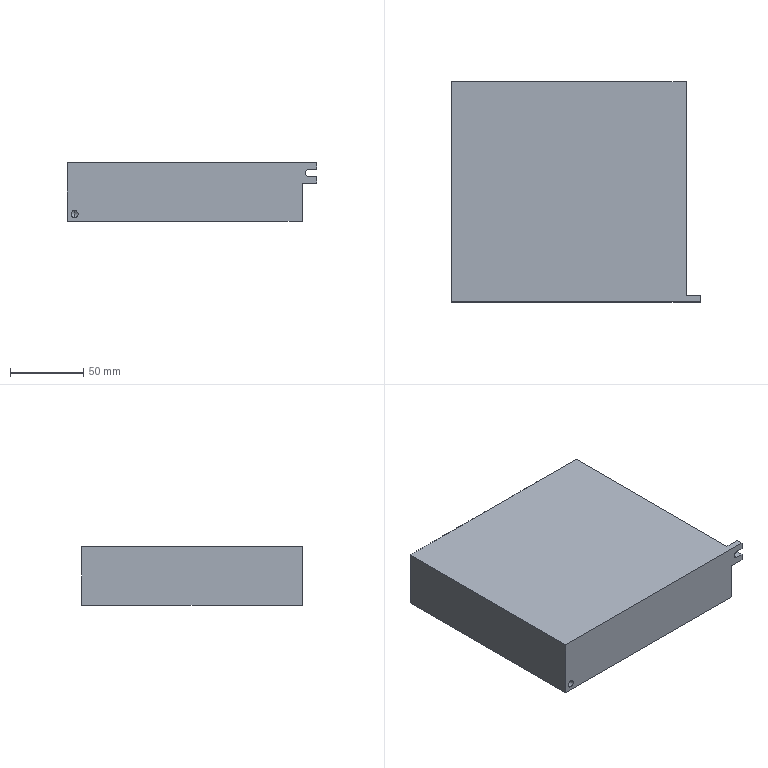Part | STEP file | Jiemeikang 400W driver | 1 solid | 17 faces | box 170 x 150 x 40 mm | volume 960193 mm3 | plane 12 | cylinder 3 | cone 2 | commonest cylinder face diameters 4.8 x2 5 x1
STEP:
#1=CARTESIAN_POINT('',(0.,0.,0.));
#2=DIRECTION('',(0.,0.,1.));
#3=DIRECTION('',(1.,0.,0.));
#4=AXIS2_PLACEMENT_3D('',#1,#2,#3);
#5=CARTESIAN_POINT('',(-75.,15.,-17.4));
#6=VERTEX_POINT('',#5);
#7=CARTESIAN_POINT('',(-75.,0.,-17.4));
#8=VERTEX_POINT('',#7);
#9=CARTESIAN_POINT('',(-75.,0.,-17.4));
#10=DIRECTION('',(0.,-1.,0.));
#11=VECTOR('',#10,1.);
#12=LINE('',#9,#11);
#13=CARTESIAN_POINT('',(-75.,0.,-15.));
#14=DIRECTION('',(0.,-1.,0.));
#15=DIRECTION('',(0.,0.,-1.));
#16=AXIS2_PLACEMENT_3D('',#13,#14,#15);
#17=CYLINDRICAL_SURFACE('',#16,2.4);
#18=CARTESIAN_POINT('',(6.283,0.));
#19=DIRECTION('',(0.,1.));
#20=VECTOR('',#19,1.);
#21=LINE('',#18,#20);
#22=(GEOMETRIC_REPRESENTATION_CONTEXT(2)PARAMETRIC_REPRESENTATION_CONTEXT()REPRESENTATION_CONTEXT('',''));
#23=DEFINITIONAL_REPRESENTATION('',(#21),#22);
#24=PCURVE('',#17,#23);
#25=CARTESIAN_POINT('',(-75.,0.,-15.));
#26=DIRECTION('',(0.,-1.,0.));
#27=DIRECTION('',(0.,0.,-1.));
#28=AXIS2_PLACEMENT_3D('',#25,#26,#27);
#29=CYLINDRICAL_SURFACE('',#28,2.4);
#30=CARTESIAN_POINT('',(0.,0.));
#31=DIRECTION('',(0.,1.));
#32=VECTOR('',#31,1.);
#33=LINE('',#30,#32);
#34=(GEOMETRIC_REPRESENTATION_CONTEXT(2)PARAMETRIC_REPRESENTATION_CONTEXT()REPRESENTATION_CONTEXT('',''));
#35=DEFINITIONAL_REPRESENTATION('',(#33),#34);
#36=PCURVE('',#29,#35);
#37=SURFACE_CURVE('',#12,(#24,#36),.PCURVE_S1.);
#38=EDGE_CURVE('',#6,#8,#37,.T.);
#39=ORIENTED_EDGE('',*,*,#38,.T.);
#40=CARTESIAN_POINT('',(-75.,0.,-12.6));
#41=VERTEX_POINT('',#40);
#42=CARTESIAN_POINT('',(-75.,0.,-15.));
#43=DIRECTION('',(0.,-1.,0.));
#44=DIRECTION('',(0.,0.,-1.));
#45=AXIS2_PLACEMENT_3D('',#42,#43,#44);
#46=CIRCLE('',#45,2.4);
#47=CARTESIAN_POINT('',(0.,0.));
#48=DIRECTION('',(1.,0.));
#49=VECTOR('',#48,1.);
#50=LINE('',#47,#49);
#51=(GEOMETRIC_REPRESENTATION_CONTEXT(2)PARAMETRIC_REPRESENTATION_CONTEXT()REPRESENTATION_CONTEXT('',''));
#52=DEFINITIONAL_REPRESENTATION('',(#50),#51);
#53=PCURVE('',#17,#52);
#54=CARTESIAN_POINT('',(0.,0.,0.));
#55=DIRECTION('',(0.,-1.,0.));
#56=DIRECTION('',(0.,0.,-1.));
#57=AXIS2_PLACEMENT_3D('',#54,#55,#56);
#58=PLANE('',#57);
#59=CARTESIAN_POINT('',(15.,-75.));
#60=DIRECTION('',(1.,0.));
#61=AXIS2_PLACEMENT_2D('',#59,#60);
#62=CIRCLE('',#61,2.4);
#63=(GEOMETRIC_REPRESENTATION_CONTEXT(2)PARAMETRIC_REPRESENTATION_CONTEXT()REPRESENTATION_CONTEXT('',''));
#64=DEFINITIONAL_REPRESENTATION('',(#62),#63);
#65=PCURVE('',#58,#64);
#66=SURFACE_CURVE('',#46,(#53,#65),.PCURVE_S1.);
#67=EDGE_CURVE('',#41,#8,#66,.T.);
#68=ORIENTED_EDGE('',*,*,#67,.F.);
#69=CARTESIAN_POINT('',(-75.,15.,-12.6));
#70=VERTEX_POINT('',#69);
#71=CARTESIAN_POINT('',(-75.,0.,-12.6));
#72=DIRECTION('',(0.,-1.,0.));
#73=VECTOR('',#72,1.);
#74=LINE('',#71,#73);
#75=CARTESIAN_POINT('',(3.142,0.));
#76=DIRECTION('',(0.,1.));
#77=VECTOR('',#76,1.);
#78=LINE('',#75,#77);
#79=(GEOMETRIC_REPRESENTATION_CONTEXT(2)PARAMETRIC_REPRESENTATION_CONTEXT()REPRESENTATION_CONTEXT('',''));
#80=DEFINITIONAL_REPRESENTATION('',(#78),#79);
#81=PCURVE('',#17,#80);
#82=CARTESIAN_POINT('',(3.142,0.));
#83=DIRECTION('',(0.,1.));
#84=VECTOR('',#83,1.);
#85=LINE('',#82,#84);
#86=(GEOMETRIC_REPRESENTATION_CONTEXT(2)PARAMETRIC_REPRESENTATION_CONTEXT()REPRESENTATION_CONTEXT('',''));
#87=DEFINITIONAL_REPRESENTATION('',(#85),#86);
#88=PCURVE('',#29,#87);
#89=SURFACE_CURVE('',#74,(#81,#88),.PCURVE_S1.);
#90=EDGE_CURVE('',#70,#41,#89,.T.);
#91=ORIENTED_EDGE('',*,*,#90,.F.);
#92=CARTESIAN_POINT('',(-75.,15.,-15.));
#93=DIRECTION('',(0.,-1.,0.));
#94=DIRECTION('',(0.,0.,-1.));
#95=AXIS2_PLACEMENT_3D('',#92,#93,#94);
#96=CIRCLE('',#95,2.4);
#97=CARTESIAN_POINT('',(0.,-15.));
#98=DIRECTION('',(1.,0.));
#99=VECTOR('',#98,1.);
#100=LINE('',#97,#99);
#101=(GEOMETRIC_REPRESENTATION_CONTEXT(2)PARAMETRIC_REPRESENTATION_CONTEXT()REPRESENTATION_CONTEXT('',''));
#102=DEFINITIONAL_REPRESENTATION('',(#100),#101);
#103=PCURVE('',#17,#102);
#104=CARTESIAN_POINT('',(-75.,15.,-15.));
#105=DIRECTION('',(0.,-1.,0.));
#106=DIRECTION('',(0.,0.,-1.));
#107=AXIS2_PLACEMENT_3D('',#104,#105,#106);
#108=CONICAL_SURFACE('',#107,2.4,1.03);
#109=CARTESIAN_POINT('',(0.,0.));
#110=DIRECTION('',(1.,0.));
#111=VECTOR('',#110,1.);
#112=LINE('',#109,#111);
#113=(GEOMETRIC_REPRESENTATION_CONTEXT(2)PARAMETRIC_REPRESENTATION_CONTEXT()REPRESENTATION_CONTEXT('',''));
#114=DEFINITIONAL_REPRESENTATION('',(#112),#113);
#115=PCURVE('',#108,#114);
#116=SURFACE_CURVE('',#96,(#103,#115),.PCURVE_S1.);
#117=EDGE_CURVE('',#70,#6,#116,.T.);
#118=ORIENTED_EDGE('',*,*,#117,.T.);
#119=EDGE_LOOP('',(#39,#68,#91,#118));
#120=FACE_BOUND('',#119,.F.);
#121=ADVANCED_FACE('',(#120),#17,.F.);
#122=ORIENTED_EDGE('',*,*,#117,.F.);
#123=CARTESIAN_POINT('',(-75.,16.442,-15.));
#124=VERTEX_POINT('',#123);
#125=CARTESIAN_POINT('',(-75.,15.,-12.6));
#126=DIRECTION('',(0.,-0.515,0.8572));
#127=VECTOR('',#126,1.);
#128=LINE('',#125,#127);
#129=CARTESIAN_POINT('',(3.142,-1.442));
#130=CARTESIAN_POINT('',(3.142,-1.42));
#131=CARTESIAN_POINT('',(3.142,-1.377));
#132=CARTESIAN_POINT('',(3.142,-1.311));
#133=CARTESIAN_POINT('',(3.142,-1.245));
#134=CARTESIAN_POINT('',(3.142,-1.18));
#135=CARTESIAN_POINT('',(3.142,-1.114));
#136=CARTESIAN_POINT('',(3.142,-1.049));
#137=CARTESIAN_POINT('',(3.142,-0.9832));
#138=CARTESIAN_POINT('',(3.142,-0.9177));
#139=CARTESIAN_POINT('',(3.142,-0.8521));
#140=CARTESIAN_POINT('',(3.142,-0.7866));
#141=CARTESIAN_POINT('',(3.142,-0.721));
#142=CARTESIAN_POINT('',(3.142,-0.6555));
#143=CARTESIAN_POINT('',(3.142,-0.5899));
#144=CARTESIAN_POINT('',(3.142,-0.5244));
#145=CARTESIAN_POINT('',(3.142,-0.4588));
#146=CARTESIAN_POINT('',(3.142,-0.3933));
#147=CARTESIAN_POINT('',(3.142,-0.3277));
#148=CARTESIAN_POINT('',(3.142,-0.2622));
#149=CARTESIAN_POINT('',(3.142,-0.1966));
#150=CARTESIAN_POINT('',(3.142,-0.1311));
#151=CARTESIAN_POINT('',(3.142,-0.06555));
#152=CARTESIAN_POINT('',(3.142,-0.02185));
#153=CARTESIAN_POINT('',(3.142,0.));
#154=B_SPLINE_CURVE_WITH_KNOTS('',3,(#129,#130,#131,#132,#133,#134,#135,#136,#137,#138,#139,#140,#141,#142,#143,#144,#145,#146,#147,#148,#149,#150,#151,#152,#153),.UNSPECIFIED.,.F.,.F.,(4,1,1,1,1,1,1,1,1,1,1,1,1,1,1,1,1,1,1,1,1,1,4),(-2.8,-2.673,-2.545,-2.418,-2.291,-2.164,-2.036,-1.909,-1.782,-1.654,-1.527,-1.4,-1.273,-1.145,-1.018,-0.8909,-0.7636,-0.6363,-0.5091,-0.3818,-0.2545,-0.1273,0.),.UNSPECIFIED.);
#155=(GEOMETRIC_REPRESENTATION_CONTEXT(2)PARAMETRIC_REPRESENTATION_CONTEXT()REPRESENTATION_CONTEXT('',''));
#156=DEFINITIONAL_REPRESENTATION('',(#154),#155);
#157=PCURVE('',#108,#156);
#158=CARTESIAN_POINT('',(-75.,15.,-15.));
#159=DIRECTION('',(0.,-1.,0.));
#160=DIRECTION('',(0.,0.,-1.));
#161=AXIS2_PLACEMENT_3D('',#158,#159,#160);
#162=CONICAL_SURFACE('',#161,2.4,1.03);
#163=CARTESIAN_POINT('',(3.142,-1.442));
#164=CARTESIAN_POINT('',(3.142,-1.42));
#165=CARTESIAN_POINT('',(3.142,-1.377));
#166=CARTESIAN_POINT('',(3.142,-1.311));
#167=CARTESIAN_POINT('',(3.142,-1.245));
#168=CARTESIAN_POINT('',(3.142,-1.18));
#169=CARTESIAN_POINT('',(3.142,-1.114));
#170=CARTESIAN_POINT('',(3.142,-1.049));
#171=CARTESIAN_POINT('',(3.142,-0.9832));
#172=CARTESIAN_POINT('',(3.142,-0.9177));
#173=CARTESIAN_POINT('',(3.142,-0.8521));
#174=CARTESIAN_POINT('',(3.142,-0.7866));
#175=CARTESIAN_POINT('',(3.142,-0.721));
#176=CARTESIAN_POINT('',(3.142,-0.6555));
#177=CARTESIAN_POINT('',(3.142,-0.5899));
#178=CARTESIAN_POINT('',(3.142,-0.5244));
#179=CARTESIAN_POINT('',(3.142,-0.4588));
#180=CARTESIAN_POINT('',(3.142,-0.3933));
#181=CARTESIAN_POINT('',(3.142,-0.3277));
#182=CARTESIAN_POINT('',(3.142,-0.2622));
#183=CARTESIAN_POINT('',(3.142,-0.1966));
#184=CARTESIAN_POINT('',(3.142,-0.1311));
#185=CARTESIAN_POINT('',(3.142,-0.06555));
#186=CARTESIAN_POINT('',(3.142,-0.02185));
#187=CARTESIAN_POINT('',(3.142,0.));
#188=B_SPLINE_CURVE_WITH_KNOTS('',3,(#163,#164,#165,#166,#167,#168,#169,#170,#171,#172,#173,#174,#175,#176,#177,#178,#179,#180,#181,#182,#183,#184,#185,#186,#187),.UNSPECIFIED.,.F.,.F.,(4,1,1,1,1,1,1,1,1,1,1,1,1,1,1,1,1,1,1,1,1,1,4),(-2.8,-2.673,-2.545,-2.418,-2.291,-2.164,-2.036,-1.909,-1.782,-1.654,-1.527,-1.4,-1.273,-1.145,-1.018,-0.8909,-0.7636,-0.6363,-0.5091,-0.3818,-0.2545,-0.1273,0.),.UNSPECIFIED.);
#189=(GEOMETRIC_REPRESENTATION_CONTEXT(2)PARAMETRIC_REPRESENTATION_CONTEXT()REPRESENTATION_CONTEXT('',''));
#190=DEFINITIONAL_REPRESENTATION('',(#188),#189);
#191=PCURVE('',#162,#190);
#192=SURFACE_CURVE('',#128,(#157,#191),.PCURVE_S1.);
#193=EDGE_CURVE('',#124,#70,#192,.T.);
#194=ORIENTED_EDGE('',*,*,#193,.F.);
#195=CARTESIAN_POINT('',(-75.,15.,-17.4));
#196=DIRECTION('',(0.,-0.515,-0.8572));
#197=VECTOR('',#196,1.);
#198=LINE('',#195,#197);
#199=CARTESIAN_POINT('',(6.283,0.));
#200=DIRECTION('',(0.,1.));
#201=VECTOR('',#200,1.);
#202=LINE('',#199,#201);
#203=(GEOMETRIC_REPRESENTATION_CONTEXT(2)PARAMETRIC_REPRESENTATION_CONTEXT()REPRESENTATION_CONTEXT('',''));
#204=DEFINITIONAL_REPRESENTATION('',(#202),#203);
#205=PCURVE('',#108,#204);
#206=CARTESIAN_POINT('',(0.,0.));
#207=DIRECTION('',(0.,1.));
#208=VECTOR('',#207,1.);
#209=LINE('',#206,#208);
#210=(GEOMETRIC_REPRESENTATION_CONTEXT(2)PARAMETRIC_REPRESENTATION_CONTEXT()REPRESENTATION_CONTEXT('',''));
#211=DEFINITIONAL_REPRESENTATION('',(#209),#210);
#212=PCURVE('',#162,#211);
#213=SURFACE_CURVE('',#198,(#205,#212),.PCURVE_S1.);
#214=EDGE_CURVE('',#124,#6,#213,.T.);
#215=ORIENTED_EDGE('',*,*,#214,.T.);
#216=EDGE_LOOP('',(#122,#194,#215));
#217=FACE_BOUND('',#216,.F.);
#218=ADVANCED_FACE('',(#217),#108,.F.);
#219=CARTESIAN_POINT('',(90.,0.,10.5));
#220=VERTEX_POINT('',#219);
#221=CARTESIAN_POINT('',(90.,4.5,10.5));
#222=VERTEX_POINT('',#221);
#223=CARTESIAN_POINT('',(90.,0.,10.5));
#224=DIRECTION('',(0.,1.,0.));
#225=VECTOR('',#224,1.);
#226=LINE('',#223,#225);
#227=CARTESIAN_POINT('',(90.,4.5,20.));
#228=DIRECTION('',(1.,0.,0.));
#229=DIRECTION('',(0.,0.,-1.));
#230=AXIS2_PLACEMENT_3D('',#227,#228,#229);
#231=PLANE('',#230);
#232=CARTESIAN_POINT('',(9.5,-4.5));
#233=DIRECTION('',(0.,1.));
#234=VECTOR('',#233,1.);
#235=LINE('',#232,#234);
#236=(GEOMETRIC_REPRESENTATION_CONTEXT(2)PARAMETRIC_REPRESENTATION_CONTEXT()REPRESENTATION_CONTEXT('',''));
#237=DEFINITIONAL_REPRESENTATION('',(#235),#236);
#238=PCURVE('',#231,#237);
#239=CARTESIAN_POINT('',(85.,0.,10.5));
#240=DIRECTION('',(0.,0.,-1.));
#241=DIRECTION('',(-1.,0.,0.));
#242=AXIS2_PLACEMENT_3D('',#239,#240,#241);
#243=PLANE('',#242);
#244=CARTESIAN_POINT('',(-5.,0.));
#245=DIRECTION('',(0.,1.));
#246=VECTOR('',#245,1.);
#247=LINE('',#244,#246);
#248=(GEOMETRIC_REPRESENTATION_CONTEXT(2)PARAMETRIC_REPRESENTATION_CONTEXT()REPRESENTATION_CONTEXT('',''));
#249=DEFINITIONAL_REPRESENTATION('',(#247),#248);
#250=PCURVE('',#243,#249);
#251=SURFACE_CURVE('',#226,(#238,#250),.PCURVE_S1.);
#252=EDGE_CURVE('',#220,#222,#251,.T.);
#253=ORIENTED_EDGE('',*,*,#252,.F.);
#254=CARTESIAN_POINT('',(90.,0.,6.));
#255=VERTEX_POINT('',#254);
#256=CARTESIAN_POINT('',(90.,0.,20.));
#257=DIRECTION('',(0.,0.,1.));
#258=VECTOR('',#257,1.);
#259=LINE('',#256,#258);
#260=CARTESIAN_POINT('',(0.,-4.5));
#261=DIRECTION('',(-1.,0.));
#262=VECTOR('',#261,1.);
#263=LINE('',#260,#262);
#264=(GEOMETRIC_REPRESENTATION_CONTEXT(2)PARAMETRIC_REPRESENTATION_CONTEXT()REPRESENTATION_CONTEXT('',''));
#265=DEFINITIONAL_REPRESENTATION('',(#263),#264);
#266=PCURVE('',#231,#265);
#267=CARTESIAN_POINT('',(-20.,90.));
#268=DIRECTION('',(-1.,0.));
#269=VECTOR('',#268,1.);
#270=LINE('',#267,#269);
#271=(GEOMETRIC_REPRESENTATION_CONTEXT(2)PARAMETRIC_REPRESENTATION_CONTEXT()REPRESENTATION_CONTEXT('',''));
#272=DEFINITIONAL_REPRESENTATION('',(#270),#271);
#273=PCURVE('',#58,#272);
#274=SURFACE_CURVE('',#259,(#266,#273),.PCURVE_S1.);
#275=EDGE_CURVE('',#255,#220,#274,.T.);
#276=ORIENTED_EDGE('',*,*,#275,.F.);
#277=CARTESIAN_POINT('',(90.,4.5,6.));
#278=VERTEX_POINT('',#277);
#279=CARTESIAN_POINT('',(90.,4.5,6.));
#280=DIRECTION('',(0.,-1.,0.));
#281=VECTOR('',#280,1.);
#282=LINE('',#279,#281);
#283=CARTESIAN_POINT('',(14.,0.));
#284=DIRECTION('',(0.,-1.));
#285=VECTOR('',#284,1.);
#286=LINE('',#283,#285);
#287=(GEOMETRIC_REPRESENTATION_CONTEXT(2)PARAMETRIC_REPRESENTATION_CONTEXT()REPRESENTATION_CONTEXT('',''));
#288=DEFINITIONAL_REPRESENTATION('',(#286),#287);
#289=PCURVE('',#231,#288);
#290=CARTESIAN_POINT('',(80.,4.5,6.));
#291=DIRECTION('',(0.,0.,-1.));
#292=DIRECTION('',(-1.,0.,0.));
#293=AXIS2_PLACEMENT_3D('',#290,#291,#292);
#294=PLANE('',#293);
#295=CARTESIAN_POINT('',(-10.,0.));
#296=DIRECTION('',(0.,-1.));
#297=VECTOR('',#296,1.);
#298=LINE('',#295,#297);
#299=(GEOMETRIC_REPRESENTATION_CONTEXT(2)PARAMETRIC_REPRESENTATION_CONTEXT()REPRESENTATION_CONTEXT('',''));
#300=DEFINITIONAL_REPRESENTATION('',(#298),#299);
#301=PCURVE('',#294,#300);
#302=SURFACE_CURVE('',#282,(#289,#301),.PCURVE_S1.);
#303=EDGE_CURVE('',#278,#255,#302,.T.);
#304=ORIENTED_EDGE('',*,*,#303,.F.);
#305=CARTESIAN_POINT('',(90.,4.5,20.));
#306=DIRECTION('',(0.,0.,1.));
#307=VECTOR('',#306,1.);
#308=LINE('',#305,#307);
#309=CARTESIAN_POINT('',(0.,0.));
#310=DIRECTION('',(-1.,0.));
#311=VECTOR('',#310,1.);
#312=LINE('',#309,#311);
#313=(GEOMETRIC_REPRESENTATION_CONTEXT(2)PARAMETRIC_REPRESENTATION_CONTEXT()REPRESENTATION_CONTEXT('',''));
#314=DEFINITIONAL_REPRESENTATION('',(#312),#313);
#315=PCURVE('',#231,#314);
#316=CARTESIAN_POINT('',(0.,4.5,0.));
#317=DIRECTION('',(0.,-1.,0.));
#318=DIRECTION('',(0.,0.,-1.));
#319=AXIS2_PLACEMENT_3D('',#316,#317,#318);
#320=PLANE('',#319);
#321=CARTESIAN_POINT('',(-20.,90.));
#322=DIRECTION('',(-1.,0.));
#323=VECTOR('',#322,1.);
#324=LINE('',#321,#323);
#325=(GEOMETRIC_REPRESENTATION_CONTEXT(2)PARAMETRIC_REPRESENTATION_CONTEXT()REPRESENTATION_CONTEXT('',''));
#326=DEFINITIONAL_REPRESENTATION('',(#324),#325);
#327=PCURVE('',#320,#326);
#328=SURFACE_CURVE('',#308,(#315,#327),.PCURVE_S1.);
#329=EDGE_CURVE('',#278,#222,#328,.T.);
#330=ORIENTED_EDGE('',*,*,#329,.T.);
#331=EDGE_LOOP('',(#253,#276,#304,#330));
#332=FACE_BOUND('',#331,.T.);
#333=ADVANCED_FACE('',(#332),#231,.T.);
#334=CARTESIAN_POINT('',(80.,150.,20.));
#335=VERTEX_POINT('',#334);
#336=CARTESIAN_POINT('',(80.,4.5,20.));
#337=VERTEX_POINT('',#336);
#338=CARTESIAN_POINT('',(80.,150.,20.));
#339=DIRECTION('',(0.,-1.,0.));
#340=VECTOR('',#339,1.);
#341=LINE('',#338,#340);
#342=CARTESIAN_POINT('',(80.,150.,20.));
#343=DIRECTION('',(-1.,0.,0.));
#344=DIRECTION('',(0.,0.,1.));
#345=AXIS2_PLACEMENT_3D('',#342,#343,#344);
#346=PLANE('',#345);
#347=CARTESIAN_POINT('',(0.,0.));
#348=DIRECTION('',(0.,-1.));
#349=VECTOR('',#348,1.);
#350=LINE('',#347,#349);
#351=(GEOMETRIC_REPRESENTATION_CONTEXT(2)PARAMETRIC_REPRESENTATION_CONTEXT()REPRESENTATION_CONTEXT('',''));
#352=DEFINITIONAL_REPRESENTATION('',(#350),#351);
#353=PCURVE('',#346,#352);
#354=CARTESIAN_POINT('',(-80.,150.,20.));
#355=DIRECTION('',(0.,0.,-1.));
#356=DIRECTION('',(-1.,0.,0.));
#357=AXIS2_PLACEMENT_3D('',#354,#355,#356);
#358=PLANE('',#357);
#359=CARTESIAN_POINT('',(-160.,0.));
#360=DIRECTION('',(0.,-1.));
#361=VECTOR('',#360,1.);
#362=LINE('',#359,#361);
#363=(GEOMETRIC_REPRESENTATION_CONTEXT(2)PARAMETRIC_REPRESENTATION_CONTEXT()REPRESENTATION_CONTEXT('',''));
#364=DEFINITIONAL_REPRESENTATION('',(#362),#363);
#365=PCURVE('',#358,#364);
#366=SURFACE_CURVE('',#341,(#353,#365),.PCURVE_S1.);
#367=EDGE_CURVE('',#335,#337,#366,.T.);
#368=ORIENTED_EDGE('',*,*,#367,.T.);
#369=CARTESIAN_POINT('',(80.,4.5,6.));
#370=VERTEX_POINT('',#369);
#371=CARTESIAN_POINT('',(80.,4.5,20.));
#372=DIRECTION('',(0.,0.,-1.));
#373=VECTOR('',#372,1.);
#374=LINE('',#371,#373);
#375=CARTESIAN_POINT('',(0.,-145.5));
#376=DIRECTION('',(-1.,0.));
#377=VECTOR('',#376,1.);
#378=LINE('',#375,#377);
#379=(GEOMETRIC_REPRESENTATION_CONTEXT(2)PARAMETRIC_REPRESENTATION_CONTEXT()REPRESENTATION_CONTEXT('',''));
#380=DEFINITIONAL_REPRESENTATION('',(#378),#379);
#381=PCURVE('',#346,#380);
#382=CARTESIAN_POINT('',(-20.,80.));
#383=DIRECTION('',(1.,0.));
#384=VECTOR('',#383,1.);
#385=LINE('',#382,#384);
#386=(GEOMETRIC_REPRESENTATION_CONTEXT(2)PARAMETRIC_REPRESENTATION_CONTEXT()REPRESENTATION_CONTEXT('',''));
#387=DEFINITIONAL_REPRESENTATION('',(#385),#386);
#388=PCURVE('',#320,#387);
#389=SURFACE_CURVE('',#374,(#381,#388),.PCURVE_S1.);
#390=EDGE_CURVE('',#337,#370,#389,.T.);
#391=ORIENTED_EDGE('',*,*,#390,.T.);
#392=CARTESIAN_POINT('',(80.,0.,6.));
#393=VERTEX_POINT('',#392);
#394=CARTESIAN_POINT('',(80.,4.5,6.));
#395=DIRECTION('',(0.,-1.,0.));
#396=VECTOR('',#395,1.);
#397=LINE('',#394,#396);
#398=CARTESIAN_POINT('',(-14.,-145.5));
#399=DIRECTION('',(0.,-1.));
#400=VECTOR('',#399,1.);
#401=LINE('',#398,#400);
#402=(GEOMETRIC_REPRESENTATION_CONTEXT(2)PARAMETRIC_REPRESENTATION_CONTEXT()REPRESENTATION_CONTEXT('',''));
#403=DEFINITIONAL_REPRESENTATION('',(#401),#402);
#404=PCURVE('',#346,#403);
#405=CARTESIAN_POINT('',(0.,0.));
#406=DIRECTION('',(0.,-1.));
#407=VECTOR('',#406,1.);
#408=LINE('',#405,#407);
#409=(GEOMETRIC_REPRESENTATION_CONTEXT(2)PARAMETRIC_REPRESENTATION_CONTEXT()REPRESENTATION_CONTEXT('',''));
#410=DEFINITIONAL_REPRESENTATION('',(#408),#409);
#411=PCURVE('',#294,#410);
#412=SURFACE_CURVE('',#397,(#404,#411),.PCURVE_S1.);
#413=EDGE_CURVE('',#370,#393,#412,.T.);
#414=ORIENTED_EDGE('',*,*,#413,.T.);
#415=CARTESIAN_POINT('',(80.,0.,-20.));
#416=VERTEX_POINT('',#415);
#417=CARTESIAN_POINT('',(80.,0.,20.));
#418=DIRECTION('',(0.,0.,-1.));
#419=VECTOR('',#418,1.);
#420=LINE('',#417,#419);
#421=CARTESIAN_POINT('',(0.,-150.));
#422=DIRECTION('',(-1.,0.));
#423=VECTOR('',#422,1.);
#424=LINE('',#421,#423);
#425=(GEOMETRIC_REPRESENTATION_CONTEXT(2)PARAMETRIC_REPRESENTATION_CONTEXT()REPRESENTATION_CONTEXT('',''));
#426=DEFINITIONAL_REPRESENTATION('',(#424),#425);
#427=PCURVE('',#346,#426);
#428=CARTESIAN_POINT('',(-20.,80.));
#429=DIRECTION('',(1.,0.));
#430=VECTOR('',#429,1.);
#431=LINE('',#428,#430);
#432=(GEOMETRIC_REPRESENTATION_CONTEXT(2)PARAMETRIC_REPRESENTATION_CONTEXT()REPRESENTATION_CONTEXT('',''));
#433=DEFINITIONAL_REPRESENTATION('',(#431),#432);
#434=PCURVE('',#58,#433);
#435=SURFACE_CURVE('',#420,(#427,#434),.PCURVE_S1.);
#436=EDGE_CURVE('',#393,#416,#435,.T.);
#437=ORIENTED_EDGE('',*,*,#436,.T.);
#438=CARTESIAN_POINT('',(80.,150.,-20.));
#439=VERTEX_POINT('',#438);
#440=CARTESIAN_POINT('',(80.,150.,-20.));
#441=DIRECTION('',(0.,-1.,0.));
#442=VECTOR('',#441,1.);
#443=LINE('',#440,#442);
#444=CARTESIAN_POINT('',(-40.,0.));
#445=DIRECTION('',(0.,-1.));
#446=VECTOR('',#445,1.);
#447=LINE('',#444,#446);
#448=(GEOMETRIC_REPRESENTATION_CONTEXT(2)PARAMETRIC_REPRESENTATION_CONTEXT()REPRESENTATION_CONTEXT('',''));
#449=DEFINITIONAL_REPRESENTATION('',(#447),#448);
#450=PCURVE('',#346,#449);
#451=CARTESIAN_POINT('',(-80.,150.,-20.));
#452=DIRECTION('',(0.,0.,1.));
#453=DIRECTION('',(1.,0.,0.));
#454=AXIS2_PLACEMENT_3D('',#451,#452,#453);
#455=PLANE('',#454);
#456=CARTESIAN_POINT('',(160.,0.));
#457=DIRECTION('',(0.,-1.));
#458=VECTOR('',#457,1.);
#459=LINE('',#456,#458);
#460=(GEOMETRIC_REPRESENTATION_CONTEXT(2)PARAMETRIC_REPRESENTATION_CONTEXT()REPRESENTATION_CONTEXT('',''));
#461=DEFINITIONAL_REPRESENTATION('',(#459),#460);
#462=PCURVE('',#455,#461);
#463=SURFACE_CURVE('',#443,(#450,#462),.PCURVE_S1.);
#464=EDGE_CURVE('',#439,#416,#463,.T.);
#465=ORIENTED_EDGE('',*,*,#464,.F.);
#466=CARTESIAN_POINT('',(80.,150.,20.));
#467=DIRECTION('',(0.,0.,-1.));
#468=VECTOR('',#467,1.);
#469=LINE('',#466,#468);
#470=CARTESIAN_POINT('',(0.,0.));
#471=DIRECTION('',(-1.,0.));
#472=VECTOR('',#471,1.);
#473=LINE('',#470,#472);
#474=(GEOMETRIC_REPRESENTATION_CONTEXT(2)PARAMETRIC_REPRESENTATION_CONTEXT()REPRESENTATION_CONTEXT('',''));
#475=DEFINITIONAL_REPRESENTATION('',(#473),#474);
#476=PCURVE('',#346,#475);
#477=CARTESIAN_POINT('',(0.,150.,0.));
#478=DIRECTION('',(0.,-1.,0.));
#479=DIRECTION('',(0.,0.,-1.));
#480=AXIS2_PLACEMENT_3D('',#477,#478,#479);
#481=PLANE('',#480);
#482=CARTESIAN_POINT('',(-20.,80.));
#483=DIRECTION('',(1.,0.));
#484=VECTOR('',#483,1.);
#485=LINE('',#482,#484);
#486=(GEOMETRIC_REPRESENTATION_CONTEXT(2)PARAMETRIC_REPRESENTATION_CONTEXT()REPRESENTATION_CONTEXT('',''));
#487=DEFINITIONAL_REPRESENTATION('',(#485),#486);
#488=PCURVE('',#481,#487);
#489=SURFACE_CURVE('',#469,(#476,#488),.PCURVE_S1.);
#490=EDGE_CURVE('',#335,#439,#489,.T.);
#491=ORIENTED_EDGE('',*,*,#490,.F.);
#492=EDGE_LOOP('',(#368,#391,#414,#437,#465,#491));
#493=FACE_BOUND('',#492,.T.);
#494=ADVANCED_FACE('',(#493),#346,.F.);
#495=CARTESIAN_POINT('',(-80.,0.,-20.));
#496=VERTEX_POINT('',#495);
#497=CARTESIAN_POINT('',(-80.,0.,-20.));
#498=DIRECTION('',(-1.,0.,0.));
#499=VECTOR('',#498,1.);
#500=LINE('',#497,#499);
#501=CARTESIAN_POINT('',(0.,-150.));
#502=DIRECTION('',(-1.,0.));
#503=VECTOR('',#502,1.);
#504=LINE('',#501,#503);
#505=(GEOMETRIC_REPRESENTATION_CONTEXT(2)PARAMETRIC_REPRESENTATION_CONTEXT()REPRESENTATION_CONTEXT('',''));
#506=DEFINITIONAL_REPRESENTATION('',(#504),#505);
#507=PCURVE('',#455,#506);
#508=CARTESIAN_POINT('',(20.,-80.));
#509=DIRECTION('',(0.,-1.));
#510=VECTOR('',#509,1.);
#511=LINE('',#508,#510);
#512=(GEOMETRIC_REPRESENTATION_CONTEXT(2)PARAMETRIC_REPRESENTATION_CONTEXT()REPRESENTATION_CONTEXT('',''));
#513=DEFINITIONAL_REPRESENTATION('',(#511),#512);
#514=PCURVE('',#58,#513);
#515=SURFACE_CURVE('',#500,(#507,#514),.PCURVE_S1.);
#516=EDGE_CURVE('',#416,#496,#515,.T.);
#517=ORIENTED_EDGE('',*,*,#516,.T.);
#518=CARTESIAN_POINT('',(-80.,150.,-20.));
#519=VERTEX_POINT('',#518);
#520=CARTESIAN_POINT('',(-80.,150.,-20.));
#521=DIRECTION('',(0.,-1.,0.));
#522=VECTOR('',#521,1.);
#523=LINE('',#520,#522);
#524=CARTESIAN_POINT('',(0.,0.));
#525=DIRECTION('',(0.,-1.));
#526=VECTOR('',#525,1.);
#527=LINE('',#524,#526);
#528=(GEOMETRIC_REPRESENTATION_CONTEXT(2)PARAMETRIC_REPRESENTATION_CONTEXT()REPRESENTATION_CONTEXT('',''));
#529=DEFINITIONAL_REPRESENTATION('',(#527),#528);
#530=PCURVE('',#455,#529);
#531=CARTESIAN_POINT('',(-80.,150.,20.));
#532=DIRECTION('',(1.,0.,0.));
#533=DIRECTION('',(0.,0.,-1.));
#534=AXIS2_PLACEMENT_3D('',#531,#532,#533);
#535=PLANE('',#534);
#536=CARTESIAN_POINT('',(40.,0.));
#537=DIRECTION('',(0.,-1.));
#538=VECTOR('',#537,1.);
#539=LINE('',#536,#538);
#540=(GEOMETRIC_REPRESENTATION_CONTEXT(2)PARAMETRIC_REPRESENTATION_CONTEXT()REPRESENTATION_CONTEXT('',''));
#541=DEFINITIONAL_REPRESENTATION('',(#539),#540);
#542=PCURVE('',#535,#541);
#543=SURFACE_CURVE('',#523,(#530,#542),.PCURVE_S1.);
#544=EDGE_CURVE('',#519,#496,#543,.T.);
#545=ORIENTED_EDGE('',*,*,#544,.F.);
#546=CARTESIAN_POINT('',(-80.,150.,-20.));
#547=DIRECTION('',(-1.,0.,0.));
#548=VECTOR('',#547,1.);
#549=LINE('',#546,#548);
#550=CARTESIAN_POINT('',(0.,0.));
#551=DIRECTION('',(-1.,0.));
#552=VECTOR('',#551,1.);
#553=LINE('',#550,#552);
#554=(GEOMETRIC_REPRESENTATION_CONTEXT(2)PARAMETRIC_REPRESENTATION_CONTEXT()REPRESENTATION_CONTEXT('',''));
#555=DEFINITIONAL_REPRESENTATION('',(#553),#554);
#556=PCURVE('',#455,#555);
#557=CARTESIAN_POINT('',(20.,-80.));
#558=DIRECTION('',(0.,-1.));
#559=VECTOR('',#558,1.);
#560=LINE('',#557,#559);
#561=(GEOMETRIC_REPRESENTATION_CONTEXT(2)PARAMETRIC_REPRESENTATION_CONTEXT()REPRESENTATION_CONTEXT('',''));
#562=DEFINITIONAL_REPRESENTATION('',(#560),#561);
#563=PCURVE('',#481,#562);
#564=SURFACE_CURVE('',#549,(#556,#563),.PCURVE_S1.);
#565=EDGE_CURVE('',#439,#519,#564,.T.);
#566=ORIENTED_EDGE('',*,*,#565,.F.);
#567=ORIENTED_EDGE('',*,*,#464,.T.);
#568=EDGE_LOOP('',(#517,#545,#566,#567));
#569=FACE_BOUND('',#568,.T.);
#570=ADVANCED_FACE('',(#569),#455,.F.);
#571=CARTESIAN_POINT('',(-80.,0.,20.));
#572=VERTEX_POINT('',#571);
#573=CARTESIAN_POINT('',(-80.,0.,20.));
#574=DIRECTION('',(0.,0.,1.));
#575=VECTOR('',#574,1.);
#576=LINE('',#573,#575);
#577=CARTESIAN_POINT('',(0.,-150.));
#578=DIRECTION('',(-1.,0.));
#579=VECTOR('',#578,1.);
#580=LINE('',#577,#579);
#581=(GEOMETRIC_REPRESENTATION_CONTEXT(2)PARAMETRIC_REPRESENTATION_CONTEXT()REPRESENTATION_CONTEXT('',''));
#582=DEFINITIONAL_REPRESENTATION('',(#580),#581);
#583=PCURVE('',#535,#582);
#584=CARTESIAN_POINT('',(-20.,-80.));
#585=DIRECTION('',(-1.,0.));
#586=VECTOR('',#585,1.);
#587=LINE('',#584,#586);
#588=(GEOMETRIC_REPRESENTATION_CONTEXT(2)PARAMETRIC_REPRESENTATION_CONTEXT()REPRESENTATION_CONTEXT('',''));
#589=DEFINITIONAL_REPRESENTATION('',(#587),#588);
#590=PCURVE('',#58,#589);
#591=SURFACE_CURVE('',#576,(#583,#590),.PCURVE_S1.);
#592=EDGE_CURVE('',#496,#572,#591,.T.);
#593=ORIENTED_EDGE('',*,*,#592,.T.);
#594=CARTESIAN_POINT('',(-80.,150.,20.));
#595=VERTEX_POINT('',#594);
#596=CARTESIAN_POINT('',(-80.,150.,20.));
#597=DIRECTION('',(0.,-1.,0.));
#598=VECTOR('',#597,1.);
#599=LINE('',#596,#598);
#600=CARTESIAN_POINT('',(0.,0.));
#601=DIRECTION('',(0.,-1.));
#602=VECTOR('',#601,1.);
#603=LINE('',#600,#602);
#604=(GEOMETRIC_REPRESENTATION_CONTEXT(2)PARAMETRIC_REPRESENTATION_CONTEXT()REPRESENTATION_CONTEXT('',''));
#605=DEFINITIONAL_REPRESENTATION('',(#603),#604);
#606=PCURVE('',#535,#605);
#607=CARTESIAN_POINT('',(0.,0.));
#608=DIRECTION('',(0.,-1.));
#609=VECTOR('',#608,1.);
#610=LINE('',#607,#609);
#611=(GEOMETRIC_REPRESENTATION_CONTEXT(2)PARAMETRIC_REPRESENTATION_CONTEXT()REPRESENTATION_CONTEXT('',''));
#612=DEFINITIONAL_REPRESENTATION('',(#610),#611);
#613=PCURVE('',#358,#612);
#614=SURFACE_CURVE('',#599,(#606,#613),.PCURVE_S1.);
#615=EDGE_CURVE('',#595,#572,#614,.T.);
#616=ORIENTED_EDGE('',*,*,#615,.F.);
#617=CARTESIAN_POINT('',(-80.,150.,20.));
#618=DIRECTION('',(0.,0.,1.));
#619=VECTOR('',#618,1.);
#620=LINE('',#617,#619);
#621=CARTESIAN_POINT('',(0.,0.));
#622=DIRECTION('',(-1.,0.));
#623=VECTOR('',#622,1.);
#624=LINE('',#621,#623);
#625=(GEOMETRIC_REPRESENTATION_CONTEXT(2)PARAMETRIC_REPRESENTATION_CONTEXT()REPRESENTATION_CONTEXT('',''));
#626=DEFINITIONAL_REPRESENTATION('',(#624),#625);
#627=PCURVE('',#535,#626);
#628=CARTESIAN_POINT('',(-20.,-80.));
#629=DIRECTION('',(-1.,0.));
#630=VECTOR('',#629,1.);
#631=LINE('',#628,#630);
#632=(GEOMETRIC_REPRESENTATION_CONTEXT(2)PARAMETRIC_REPRESENTATION_CONTEXT()REPRESENTATION_CONTEXT('',''));
#633=DEFINITIONAL_REPRESENTATION('',(#631),#632);
#634=PCURVE('',#481,#633);
#635=SURFACE_CURVE('',#620,(#627,#634),.PCURVE_S1.);
#636=EDGE_CURVE('',#519,#595,#635,.T.);
#637=ORIENTED_EDGE('',*,*,#636,.F.);
#638=ORIENTED_EDGE('',*,*,#544,.T.);
#639=EDGE_LOOP('',(#593,#616,#637,#638));
#640=FACE_BOUND('',#639,.T.);
#641=ADVANCED_FACE('',(#640),#535,.F.);
#642=CARTESIAN_POINT('',(90.,0.,20.));
#643=VERTEX_POINT('',#642);
#644=CARTESIAN_POINT('',(-80.,0.,20.));
#645=DIRECTION('',(1.,0.,0.));
#646=VECTOR('',#645,1.);
#647=LINE('',#644,#646);
#648=CARTESIAN_POINT('',(0.,-150.));
#649=DIRECTION('',(-1.,0.));
#650=VECTOR('',#649,1.);
#651=LINE('',#648,#650);
#652=(GEOMETRIC_REPRESENTATION_CONTEXT(2)PARAMETRIC_REPRESENTATION_CONTEXT()REPRESENTATION_CONTEXT('',''));
#653=DEFINITIONAL_REPRESENTATION('',(#651),#652);
#654=PCURVE('',#358,#653);
#655=CARTESIAN_POINT('',(-20.,-80.));
#656=DIRECTION('',(0.,1.));
#657=VECTOR('',#656,1.);
#658=LINE('',#655,#657);
#659=(GEOMETRIC_REPRESENTATION_CONTEXT(2)PARAMETRIC_REPRESENTATION_CONTEXT()REPRESENTATION_CONTEXT('',''));
#660=DEFINITIONAL_REPRESENTATION('',(#658),#659);
#661=PCURVE('',#58,#660);
#662=SURFACE_CURVE('',#647,(#654,#661),.PCURVE_S1.);
#663=EDGE_CURVE('',#572,#643,#662,.T.);
#664=ORIENTED_EDGE('',*,*,#663,.T.);
#665=CARTESIAN_POINT('',(90.,4.5,20.));
#666=VERTEX_POINT('',#665);
#667=CARTESIAN_POINT('',(90.,4.5,20.));
#668=DIRECTION('',(0.,-1.,0.));
#669=VECTOR('',#668,1.);
#670=LINE('',#667,#669);
#671=CARTESIAN_POINT('',(-170.,-145.5));
#672=DIRECTION('',(0.,-1.));
#673=VECTOR('',#672,1.);
#674=LINE('',#671,#673);
#675=(GEOMETRIC_REPRESENTATION_CONTEXT(2)PARAMETRIC_REPRESENTATION_CONTEXT()REPRESENTATION_CONTEXT('',''));
#676=DEFINITIONAL_REPRESENTATION('',(#674),#675);
#677=PCURVE('',#358,#676);
#678=CARTESIAN_POINT('',(90.,4.5,20.));
#679=DIRECTION('',(1.,0.,0.));
#680=DIRECTION('',(0.,0.,-1.));
#681=AXIS2_PLACEMENT_3D('',#678,#679,#680);
#682=PLANE('',#681);
#683=CARTESIAN_POINT('',(0.,0.));
#684=DIRECTION('',(0.,-1.));
#685=VECTOR('',#684,1.);
#686=LINE('',#683,#685);
#687=(GEOMETRIC_REPRESENTATION_CONTEXT(2)PARAMETRIC_REPRESENTATION_CONTEXT()REPRESENTATION_CONTEXT('',''));
#688=DEFINITIONAL_REPRESENTATION('',(#686),#687);
#689=PCURVE('',#682,#688);
#690=SURFACE_CURVE('',#670,(#677,#689),.PCURVE_S1.);
#691=EDGE_CURVE('',#666,#643,#690,.T.);
#692=ORIENTED_EDGE('',*,*,#691,.F.);
#693=CARTESIAN_POINT('',(80.,4.5,20.));
#694=DIRECTION('',(-1.,0.,0.));
#695=VECTOR('',#694,1.);
#696=LINE('',#693,#695);
#697=CARTESIAN_POINT('',(-160.,-145.5));
#698=DIRECTION('',(1.,0.));
#699=VECTOR('',#698,1.);
#700=LINE('',#697,#699);
#701=(GEOMETRIC_REPRESENTATION_CONTEXT(2)PARAMETRIC_REPRESENTATION_CONTEXT()REPRESENTATION_CONTEXT('',''));
#702=DEFINITIONAL_REPRESENTATION('',(#700),#701);
#703=PCURVE('',#358,#702);
#704=CARTESIAN_POINT('',(-20.,80.));
#705=DIRECTION('',(0.,-1.));
#706=VECTOR('',#705,1.);
#707=LINE('',#704,#706);
#708=(GEOMETRIC_REPRESENTATION_CONTEXT(2)PARAMETRIC_REPRESENTATION_CONTEXT()REPRESENTATION_CONTEXT('',''));
#709=DEFINITIONAL_REPRESENTATION('',(#707),#708);
#710=PCURVE('',#320,#709);
#711=SURFACE_CURVE('',#696,(#703,#710),.PCURVE_S1.);
#712=EDGE_CURVE('',#666,#337,#711,.T.);
#713=ORIENTED_EDGE('',*,*,#712,.T.);
#714=ORIENTED_EDGE('',*,*,#367,.F.);
#715=CARTESIAN_POINT('',(-80.,150.,20.));
#716=DIRECTION('',(1.,0.,0.));
#717=VECTOR('',#716,1.);
#718=LINE('',#715,#717);
#719=CARTESIAN_POINT('',(0.,0.));
#720=DIRECTION('',(-1.,0.));
#721=VECTOR('',#720,1.);
#722=LINE('',#719,#721);
#723=(GEOMETRIC_REPRESENTATION_CONTEXT(2)PARAMETRIC_REPRESENTATION_CONTEXT()REPRESENTATION_CONTEXT('',''));
#724=DEFINITIONAL_REPRESENTATION('',(#722),#723);
#725=PCURVE('',#358,#724);
#726=CARTESIAN_POINT('',(-20.,-80.));
#727=DIRECTION('',(0.,1.));
#728=VECTOR('',#727,1.);
#729=LINE('',#726,#728);
#730=(GEOMETRIC_REPRESENTATION_CONTEXT(2)PARAMETRIC_REPRESENTATION_CONTEXT()REPRESENTATION_CONTEXT('',''));
#731=DEFINITIONAL_REPRESENTATION('',(#729),#730);
#732=PCURVE('',#481,#731);
#733=SURFACE_CURVE('',#718,(#725,#732),.PCURVE_S1.);
#734=EDGE_CURVE('',#595,#335,#733,.T.);
#735=ORIENTED_EDGE('',*,*,#734,.F.);
#736=ORIENTED_EDGE('',*,*,#615,.T.);
#737=EDGE_LOOP('',(#664,#692,#713,#714,#735,#736));
#738=FACE_BOUND('',#737,.T.);
#739=ADVANCED_FACE('',(#738),#358,.F.);
#740=ORIENTED_EDGE('',*,*,#490,.T.);
#741=ORIENTED_EDGE('',*,*,#565,.T.);
#742=ORIENTED_EDGE('',*,*,#636,.T.);
#743=ORIENTED_EDGE('',*,*,#734,.T.);
#744=EDGE_LOOP('',(#740,#741,#742,#743));
#745=FACE_BOUND('',#744,.T.);
#746=ADVANCED_FACE('',(#745),#481,.F.);
#747=CARTESIAN_POINT('',(85.,0.,10.5));
#748=VERTEX_POINT('',#747);
#749=CARTESIAN_POINT('',(85.,0.,10.5));
#750=DIRECTION('',(-1.,0.,0.));
#751=VECTOR('',#750,1.);
#752=LINE('',#749,#751);
#753=CARTESIAN_POINT('',(-10.5,85.));
#754=DIRECTION('',(0.,-1.));
#755=VECTOR('',#754,1.);
#756=LINE('',#753,#755);
#757=(GEOMETRIC_REPRESENTATION_CONTEXT(2)PARAMETRIC_REPRESENTATION_CONTEXT()REPRESENTATION_CONTEXT('',''));
#758=DEFINITIONAL_REPRESENTATION('',(#756),#757);
#759=PCURVE('',#58,#758);
#760=CARTESIAN_POINT('',(0.,0.));
#761=DIRECTION('',(1.,0.));
#762=VECTOR('',#761,1.);
#763=LINE('',#760,#762);
#764=(GEOMETRIC_REPRESENTATION_CONTEXT(2)PARAMETRIC_REPRESENTATION_CONTEXT()REPRESENTATION_CONTEXT('',''));
#765=DEFINITIONAL_REPRESENTATION('',(#763),#764);
#766=PCURVE('',#243,#765);
#767=SURFACE_CURVE('',#752,(#759,#766),.PCURVE_S1.);
#768=EDGE_CURVE('',#220,#748,#767,.T.);
#769=ORIENTED_EDGE('',*,*,#768,.T.);
#770=CARTESIAN_POINT('',(85.,0.,15.5));
#771=VERTEX_POINT('',#770);
#772=CARTESIAN_POINT('',(85.,0.,13.));
#773=DIRECTION('',(0.,1.,0.));
#774=DIRECTION('',(0.,0.,1.));
#775=AXIS2_PLACEMENT_3D('',#772,#773,#774);
#776=CIRCLE('',#775,2.5);
#777=CARTESIAN_POINT('',(-15.5,85.));
#778=CARTESIAN_POINT('',(-15.5,89.33));
#779=CARTESIAN_POINT('',(-11.75,87.165));
#780=CARTESIAN_POINT('',(-8.,85.));
#781=CARTESIAN_POINT('',(-11.75,82.835));
#782=CARTESIAN_POINT('',(-15.5,80.67));
#783=CARTESIAN_POINT('',(-15.5,85.));
#784=(BOUNDED_CURVE()B_SPLINE_CURVE(2,(#777,#778,#779,#780,#781,#782,#783),.UNSPECIFIED.,.T.,.F.)B_SPLINE_CURVE_WITH_KNOTS((1,2,2,2,2,1),(-2.094,0.,2.094,4.189,6.283,8.378),.UNSPECIFIED.)CURVE()GEOMETRIC_REPRESENTATION_ITEM()RATIONAL_B_SPLINE_CURVE((1.,0.5,1.,0.5,1.,0.5,1.))REPRESENTATION_ITEM(''));
#785=(GEOMETRIC_REPRESENTATION_CONTEXT(2)PARAMETRIC_REPRESENTATION_CONTEXT()REPRESENTATION_CONTEXT('',''));
#786=DEFINITIONAL_REPRESENTATION('',(#784),#785);
#787=PCURVE('',#58,#786);
#788=CARTESIAN_POINT('',(85.,0.,13.));
#789=DIRECTION('',(0.,1.,0.));
#790=DIRECTION('',(0.,0.,1.));
#791=AXIS2_PLACEMENT_3D('',#788,#789,#790);
#792=CYLINDRICAL_SURFACE('',#791,2.5);
#793=CARTESIAN_POINT('',(0.,0.));
#794=DIRECTION('',(1.,0.));
#795=VECTOR('',#794,1.);
#796=LINE('',#793,#795);
#797=(GEOMETRIC_REPRESENTATION_CONTEXT(2)PARAMETRIC_REPRESENTATION_CONTEXT()REPRESENTATION_CONTEXT('',''));
#798=DEFINITIONAL_REPRESENTATION('',(#796),#797);
#799=PCURVE('',#792,#798);
#800=SURFACE_CURVE('',#776,(#787,#799),.PCURVE_S1.);
#801=EDGE_CURVE('',#748,#771,#800,.T.);
#802=ORIENTED_EDGE('',*,*,#801,.T.);
#803=CARTESIAN_POINT('',(90.,0.,15.5));
#804=VERTEX_POINT('',#803);
#805=CARTESIAN_POINT('',(85.,0.,15.5));
#806=DIRECTION('',(1.,0.,0.));
#807=VECTOR('',#806,1.);
#808=LINE('',#805,#807);
#809=CARTESIAN_POINT('',(-15.5,85.));
#810=DIRECTION('',(0.,1.));
#811=VECTOR('',#810,1.);
#812=LINE('',#809,#811);
#813=(GEOMETRIC_REPRESENTATION_CONTEXT(2)PARAMETRIC_REPRESENTATION_CONTEXT()REPRESENTATION_CONTEXT('',''));
#814=DEFINITIONAL_REPRESENTATION('',(#812),#813);
#815=PCURVE('',#58,#814);
#816=CARTESIAN_POINT('',(85.,0.,15.5));
#817=DIRECTION('',(0.,0.,1.));
#818=DIRECTION('',(1.,0.,0.));
#819=AXIS2_PLACEMENT_3D('',#816,#817,#818);
#820=PLANE('',#819);
#821=CARTESIAN_POINT('',(0.,0.));
#822=DIRECTION('',(1.,0.));
#823=VECTOR('',#822,1.);
#824=LINE('',#821,#823);
#825=(GEOMETRIC_REPRESENTATION_CONTEXT(2)PARAMETRIC_REPRESENTATION_CONTEXT()REPRESENTATION_CONTEXT('',''));
#826=DEFINITIONAL_REPRESENTATION('',(#824),#825);
#827=PCURVE('',#820,#826);
#828=SURFACE_CURVE('',#808,(#815,#827),.PCURVE_S1.);
#829=EDGE_CURVE('',#771,#804,#828,.T.);
#830=ORIENTED_EDGE('',*,*,#829,.T.);
#831=CARTESIAN_POINT('',(90.,0.,20.));
#832=DIRECTION('',(0.,0.,1.));
#833=VECTOR('',#832,1.);
#834=LINE('',#831,#833);
#835=CARTESIAN_POINT('',(-20.,90.));
#836=DIRECTION('',(-1.,0.));
#837=VECTOR('',#836,1.);
#838=LINE('',#835,#837);
#839=(GEOMETRIC_REPRESENTATION_CONTEXT(2)PARAMETRIC_REPRESENTATION_CONTEXT()REPRESENTATION_CONTEXT('',''));
#840=DEFINITIONAL_REPRESENTATION('',(#838),#839);
#841=PCURVE('',#58,#840);
#842=CARTESIAN_POINT('',(0.,-4.5));
#843=DIRECTION('',(-1.,0.));
#844=VECTOR('',#843,1.);
#845=LINE('',#842,#844);
#846=(GEOMETRIC_REPRESENTATION_CONTEXT(2)PARAMETRIC_REPRESENTATION_CONTEXT()REPRESENTATION_CONTEXT('',''));
#847=DEFINITIONAL_REPRESENTATION('',(#845),#846);
#848=PCURVE('',#682,#847);
#849=SURFACE_CURVE('',#834,(#841,#848),.PCURVE_S1.);
#850=EDGE_CURVE('',#804,#643,#849,.T.);
#851=ORIENTED_EDGE('',*,*,#850,.T.);
#852=ORIENTED_EDGE('',*,*,#663,.F.);
#853=ORIENTED_EDGE('',*,*,#592,.F.);
#854=ORIENTED_EDGE('',*,*,#516,.F.);
#855=ORIENTED_EDGE('',*,*,#436,.F.);
#856=CARTESIAN_POINT('',(80.,0.,6.));
#857=DIRECTION('',(1.,0.,0.));
#858=VECTOR('',#857,1.);
#859=LINE('',#856,#858);
#860=CARTESIAN_POINT('',(-6.,80.));
#861=DIRECTION('',(0.,1.));
#862=VECTOR('',#861,1.);
#863=LINE('',#860,#862);
#864=(GEOMETRIC_REPRESENTATION_CONTEXT(2)PARAMETRIC_REPRESENTATION_CONTEXT()REPRESENTATION_CONTEXT('',''));
#865=DEFINITIONAL_REPRESENTATION('',(#863),#864);
#866=PCURVE('',#58,#865);
#867=CARTESIAN_POINT('',(0.,-4.5));
#868=DIRECTION('',(-1.,0.));
#869=VECTOR('',#868,1.);
#870=LINE('',#867,#869);
#871=(GEOMETRIC_REPRESENTATION_CONTEXT(2)PARAMETRIC_REPRESENTATION_CONTEXT()REPRESENTATION_CONTEXT('',''));
#872=DEFINITIONAL_REPRESENTATION('',(#870),#871);
#873=PCURVE('',#294,#872);
#874=SURFACE_CURVE('',#859,(#866,#873),.PCURVE_S1.);
#875=EDGE_CURVE('',#393,#255,#874,.T.);
#876=ORIENTED_EDGE('',*,*,#875,.T.);
#877=ORIENTED_EDGE('',*,*,#275,.T.);
#878=EDGE_LOOP('',(#769,#802,#830,#851,#852,#853,#854,#855,#876,#877));
#879=FACE_BOUND('',#878,.T.);
#880=CARTESIAN_POINT('',(-75.,0.,-15.));
#881=DIRECTION('',(0.,-1.,0.));
#882=DIRECTION('',(0.,0.,-1.));
#883=AXIS2_PLACEMENT_3D('',#880,#881,#882);
#884=CIRCLE('',#883,2.4);
#885=CARTESIAN_POINT('',(15.,-75.));
#886=DIRECTION('',(1.,0.));
#887=AXIS2_PLACEMENT_2D('',#885,#886);
#888=CIRCLE('',#887,2.4);
#889=(GEOMETRIC_REPRESENTATION_CONTEXT(2)PARAMETRIC_REPRESENTATION_CONTEXT()REPRESENTATION_CONTEXT('',''));
#890=DEFINITIONAL_REPRESENTATION('',(#888),#889);
#891=PCURVE('',#58,#890);
#892=CARTESIAN_POINT('',(0.,0.));
#893=DIRECTION('',(1.,0.));
#894=VECTOR('',#893,1.);
#895=LINE('',#892,#894);
#896=(GEOMETRIC_REPRESENTATION_CONTEXT(2)PARAMETRIC_REPRESENTATION_CONTEXT()REPRESENTATION_CONTEXT('',''));
#897=DEFINITIONAL_REPRESENTATION('',(#895),#896);
#898=PCURVE('',#29,#897);
#899=SURFACE_CURVE('',#884,(#891,#898),.PCURVE_S1.);
#900=EDGE_CURVE('',#8,#41,#899,.T.);
#901=ORIENTED_EDGE('',*,*,#900,.F.);
#902=ORIENTED_EDGE('',*,*,#67,.F.);
#903=EDGE_LOOP('',(#901,#902));
#904=FACE_BOUND('',#903,.T.);
#905=ADVANCED_FACE('',(#879,#904),#58,.T.);
#906=CARTESIAN_POINT('',(90.,4.5,15.5));
#907=VERTEX_POINT('',#906);
#908=CARTESIAN_POINT('',(90.,0.,15.5));
#909=DIRECTION('',(0.,1.,0.));
#910=VECTOR('',#909,1.);
#911=LINE('',#908,#910);
#912=CARTESIAN_POINT('',(4.5,-4.5));
#913=DIRECTION('',(0.,1.));
#914=VECTOR('',#913,1.);
#915=LINE('',#912,#914);
#916=(GEOMETRIC_REPRESENTATION_CONTEXT(2)PARAMETRIC_REPRESENTATION_CONTEXT()REPRESENTATION_CONTEXT('',''));
#917=DEFINITIONAL_REPRESENTATION('',(#915),#916);
#918=PCURVE('',#682,#917);
#919=CARTESIAN_POINT('',(5.,0.));
#920=DIRECTION('',(0.,1.));
#921=VECTOR('',#920,1.);
#922=LINE('',#919,#921);
#923=(GEOMETRIC_REPRESENTATION_CONTEXT(2)PARAMETRIC_REPRESENTATION_CONTEXT()REPRESENTATION_CONTEXT('',''));
#924=DEFINITIONAL_REPRESENTATION('',(#922),#923);
#925=PCURVE('',#820,#924);
#926=SURFACE_CURVE('',#911,(#918,#925),.PCURVE_S1.);
#927=EDGE_CURVE('',#804,#907,#926,.T.);
#928=ORIENTED_EDGE('',*,*,#927,.T.);
#929=CARTESIAN_POINT('',(90.,4.5,20.));
#930=DIRECTION('',(0.,0.,1.));
#931=VECTOR('',#930,1.);
#932=LINE('',#929,#931);
#933=CARTESIAN_POINT('',(0.,0.));
#934=DIRECTION('',(-1.,0.));
#935=VECTOR('',#934,1.);
#936=LINE('',#933,#935);
#937=(GEOMETRIC_REPRESENTATION_CONTEXT(2)PARAMETRIC_REPRESENTATION_CONTEXT()REPRESENTATION_CONTEXT('',''));
#938=DEFINITIONAL_REPRESENTATION('',(#936),#937);
#939=PCURVE('',#682,#938);
#940=CARTESIAN_POINT('',(-20.,90.));
#941=DIRECTION('',(-1.,0.));
#942=VECTOR('',#941,1.);
#943=LINE('',#940,#942);
#944=(GEOMETRIC_REPRESENTATION_CONTEXT(2)PARAMETRIC_REPRESENTATION_CONTEXT()REPRESENTATION_CONTEXT('',''));
#945=DEFINITIONAL_REPRESENTATION('',(#943),#944);
#946=PCURVE('',#320,#945);
#947=SURFACE_CURVE('',#932,(#939,#946),.PCURVE_S1.);
#948=EDGE_CURVE('',#907,#666,#947,.T.);
#949=ORIENTED_EDGE('',*,*,#948,.T.);
#950=ORIENTED_EDGE('',*,*,#691,.T.);
#951=ORIENTED_EDGE('',*,*,#850,.F.);
#952=EDGE_LOOP('',(#928,#949,#950,#951));
#953=FACE_BOUND('',#952,.T.);
#954=ADVANCED_FACE('',(#953),#682,.T.);
#955=ORIENTED_EDGE('',*,*,#875,.F.);
#956=ORIENTED_EDGE('',*,*,#413,.F.);
#957=CARTESIAN_POINT('',(80.,4.5,6.));
#958=DIRECTION('',(1.,0.,0.));
#959=VECTOR('',#958,1.);
#960=LINE('',#957,#959);
#961=CARTESIAN_POINT('',(0.,0.));
#962=DIRECTION('',(-1.,0.));
#963=VECTOR('',#962,1.);
#964=LINE('',#961,#963);
#965=(GEOMETRIC_REPRESENTATION_CONTEXT(2)PARAMETRIC_REPRESENTATION_CONTEXT()REPRESENTATION_CONTEXT('',''));
#966=DEFINITIONAL_REPRESENTATION('',(#964),#965);
#967=PCURVE('',#294,#966);
#968=CARTESIAN_POINT('',(-6.,80.));
#969=DIRECTION('',(0.,1.));
#970=VECTOR('',#969,1.);
#971=LINE('',#968,#970);
#972=(GEOMETRIC_REPRESENTATION_CONTEXT(2)PARAMETRIC_REPRESENTATION_CONTEXT()REPRESENTATION_CONTEXT('',''));
#973=DEFINITIONAL_REPRESENTATION('',(#971),#972);
#974=PCURVE('',#320,#973);
#975=SURFACE_CURVE('',#960,(#967,#974),.PCURVE_S1.);
#976=EDGE_CURVE('',#370,#278,#975,.T.);
#977=ORIENTED_EDGE('',*,*,#976,.T.);
#978=ORIENTED_EDGE('',*,*,#303,.T.);
#979=EDGE_LOOP('',(#955,#956,#977,#978));
#980=FACE_BOUND('',#979,.T.);
#981=ADVANCED_FACE('',(#980),#294,.T.);
#982=CARTESIAN_POINT('',(85.,4.5,10.5));
#983=VERTEX_POINT('',#982);
#984=CARTESIAN_POINT('',(85.,4.5,15.5));
#985=VERTEX_POINT('',#984);
#986=CARTESIAN_POINT('',(85.,4.5,13.));
#987=DIRECTION('',(0.,1.,0.));
#988=DIRECTION('',(0.,0.,1.));
#989=AXIS2_PLACEMENT_3D('',#986,#987,#988);
#990=CIRCLE('',#989,2.5);
#991=CARTESIAN_POINT('',(-15.5,85.));
#992=CARTESIAN_POINT('',(-15.5,89.33));
#993=CARTESIAN_POINT('',(-11.75,87.165));
#994=CARTESIAN_POINT('',(-8.,85.));
#995=CARTESIAN_POINT('',(-11.75,82.835));
#996=CARTESIAN_POINT('',(-15.5,80.67));
#997=CARTESIAN_POINT('',(-15.5,85.));
#998=(BOUNDED_CURVE()B_SPLINE_CURVE(2,(#991,#992,#993,#994,#995,#996,#997),.UNSPECIFIED.,.T.,.F.)B_SPLINE_CURVE_WITH_KNOTS((1,2,2,2,2,1),(-2.094,0.,2.094,4.189,6.283,8.378),.UNSPECIFIED.)CURVE()GEOMETRIC_REPRESENTATION_ITEM()RATIONAL_B_SPLINE_CURVE((1.,0.5,1.,0.5,1.,0.5,1.))REPRESENTATION_ITEM(''));
#999=(GEOMETRIC_REPRESENTATION_CONTEXT(2)PARAMETRIC_REPRESENTATION_CONTEXT()REPRESENTATION_CONTEXT('',''));
#1000=DEFINITIONAL_REPRESENTATION('',(#998),#999);
#1001=PCURVE('',#320,#1000);
#1002=CARTESIAN_POINT('',(0.,4.5));
#1003=DIRECTION('',(1.,0.));
#1004=VECTOR('',#1003,1.);
#1005=LINE('',#1002,#1004);
#1006=(GEOMETRIC_REPRESENTATION_CONTEXT(2)PARAMETRIC_REPRESENTATION_CONTEXT()REPRESENTATION_CONTEXT('',''));
#1007=DEFINITIONAL_REPRESENTATION('',(#1005),#1006);
#1008=PCURVE('',#792,#1007);
#1009=SURFACE_CURVE('',#990,(#1001,#1008),.PCURVE_S1.);
#1010=EDGE_CURVE('',#983,#985,#1009,.T.);
#1011=ORIENTED_EDGE('',*,*,#1010,.F.);
#1012=CARTESIAN_POINT('',(85.,4.5,10.5));
#1013=DIRECTION('',(-1.,0.,0.));
#1014=VECTOR('',#1013,1.);
#1015=LINE('',#1012,#1014);
#1016=CARTESIAN_POINT('',(-10.5,85.));
#1017=DIRECTION('',(0.,-1.));
#1018=VECTOR('',#1017,1.);
#1019=LINE('',#1016,#1018);
#1020=(GEOMETRIC_REPRESENTATION_CONTEXT(2)PARAMETRIC_REPRESENTATION_CONTEXT()REPRESENTATION_CONTEXT('',''));
#1021=DEFINITIONAL_REPRESENTATION('',(#1019),#1020);
#1022=PCURVE('',#320,#1021);
#1023=CARTESIAN_POINT('',(0.,4.5));
#1024=DIRECTION('',(1.,0.));
#1025=VECTOR('',#1024,1.);
#1026=LINE('',#1023,#1025);
#1027=(GEOMETRIC_REPRESENTATION_CONTEXT(2)PARAMETRIC_REPRESENTATION_CONTEXT()REPRESENTATION_CONTEXT('',''));
#1028=DEFINITIONAL_REPRESENTATION('',(#1026),#1027);
#1029=PCURVE('',#243,#1028);
#1030=SURFACE_CURVE('',#1015,(#1022,#1029),.PCURVE_S1.);
#1031=EDGE_CURVE('',#222,#983,#1030,.T.);
#1032=ORIENTED_EDGE('',*,*,#1031,.F.);
#1033=ORIENTED_EDGE('',*,*,#329,.F.);
#1034=ORIENTED_EDGE('',*,*,#976,.F.);
#1035=ORIENTED_EDGE('',*,*,#390,.F.);
#1036=ORIENTED_EDGE('',*,*,#712,.F.);
#1037=ORIENTED_EDGE('',*,*,#948,.F.);
#1038=CARTESIAN_POINT('',(85.,4.5,15.5));
#1039=DIRECTION('',(1.,0.,0.));
#1040=VECTOR('',#1039,1.);
#1041=LINE('',#1038,#1040);
#1042=CARTESIAN_POINT('',(-15.5,85.));
#1043=DIRECTION('',(0.,1.));
#1044=VECTOR('',#1043,1.);
#1045=LINE('',#1042,#1044);
#1046=(GEOMETRIC_REPRESENTATION_CONTEXT(2)PARAMETRIC_REPRESENTATION_CONTEXT()REPRESENTATION_CONTEXT('',''));
#1047=DEFINITIONAL_REPRESENTATION('',(#1045),#1046);
#1048=PCURVE('',#320,#1047);
#1049=CARTESIAN_POINT('',(0.,4.5));
#1050=DIRECTION('',(1.,0.));
#1051=VECTOR('',#1050,1.);
#1052=LINE('',#1049,#1051);
#1053=(GEOMETRIC_REPRESENTATION_CONTEXT(2)PARAMETRIC_REPRESENTATION_CONTEXT()REPRESENTATION_CONTEXT('',''));
#1054=DEFINITIONAL_REPRESENTATION('',(#1052),#1053);
#1055=PCURVE('',#820,#1054);
#1056=SURFACE_CURVE('',#1041,(#1048,#1055),.PCURVE_S1.);
#1057=EDGE_CURVE('',#985,#907,#1056,.T.);
#1058=ORIENTED_EDGE('',*,*,#1057,.F.);
#1059=EDGE_LOOP('',(#1011,#1032,#1033,#1034,#1035,#1036,#1037,#1058));
#1060=FACE_BOUND('',#1059,.T.);
#1061=ADVANCED_FACE('',(#1060),#320,.F.);
#1062=CARTESIAN_POINT('',(-75.,15.,-15.));
#1063=DIRECTION('',(0.,-1.,0.));
#1064=DIRECTION('',(0.,0.,-1.));
#1065=AXIS2_PLACEMENT_3D('',#1062,#1063,#1064);
#1066=CIRCLE('',#1065,2.4);
#1067=CARTESIAN_POINT('',(0.,0.));
#1068=DIRECTION('',(1.,0.));
#1069=VECTOR('',#1068,1.);
#1070=LINE('',#1067,#1069);
#1071=(GEOMETRIC_REPRESENTATION_CONTEXT(2)PARAMETRIC_REPRESENTATION_CONTEXT()REPRESENTATION_CONTEXT('',''));
#1072=DEFINITIONAL_REPRESENTATION('',(#1070),#1071);
#1073=PCURVE('',#162,#1072);
#1074=CARTESIAN_POINT('',(0.,-15.));
#1075=DIRECTION('',(1.,0.));
#1076=VECTOR('',#1075,1.);
#1077=LINE('',#1074,#1076);
#1078=(GEOMETRIC_REPRESENTATION_CONTEXT(2)PARAMETRIC_REPRESENTATION_CONTEXT()REPRESENTATION_CONTEXT('',''));
#1079=DEFINITIONAL_REPRESENTATION('',(#1077),#1078);
#1080=PCURVE('',#29,#1079);
#1081=SURFACE_CURVE('',#1066,(#1073,#1080),.PCURVE_S1.);
#1082=EDGE_CURVE('',#6,#70,#1081,.T.);
#1083=ORIENTED_EDGE('',*,*,#1082,.F.);
#1084=ORIENTED_EDGE('',*,*,#214,.F.);
#1085=ORIENTED_EDGE('',*,*,#193,.T.);
#1086=EDGE_LOOP('',(#1083,#1084,#1085));
#1087=FACE_BOUND('',#1086,.F.);
#1088=ADVANCED_FACE('',(#1087),#162,.F.);
#1089=ORIENTED_EDGE('',*,*,#900,.F.);
#1090=ORIENTED_EDGE('',*,*,#38,.F.);
#1091=ORIENTED_EDGE('',*,*,#1082,.T.);
#1092=ORIENTED_EDGE('',*,*,#90,.T.);
#1093=EDGE_LOOP('',(#1089,#1090,#1091,#1092));
#1094=FACE_BOUND('',#1093,.F.);
#1095=ADVANCED_FACE('',(#1094),#29,.F.);
#1096=CARTESIAN_POINT('',(85.,0.,10.5));
#1097=DIRECTION('',(0.,1.,0.));
#1098=VECTOR('',#1097,1.);
#1099=LINE('',#1096,#1098);
#1100=CARTESIAN_POINT('',(3.142,0.));
#1101=DIRECTION('',(0.,1.));
#1102=VECTOR('',#1101,1.);
#1103=LINE('',#1100,#1102);
#1104=(GEOMETRIC_REPRESENTATION_CONTEXT(2)PARAMETRIC_REPRESENTATION_CONTEXT()REPRESENTATION_CONTEXT('',''));
#1105=DEFINITIONAL_REPRESENTATION('',(#1103),#1104);
#1106=PCURVE('',#792,#1105);
#1107=CARTESIAN_POINT('',(0.,0.));
#1108=DIRECTION('',(0.,1.));
#1109=VECTOR('',#1108,1.);
#1110=LINE('',#1107,#1109);
#1111=(GEOMETRIC_REPRESENTATION_CONTEXT(2)PARAMETRIC_REPRESENTATION_CONTEXT()REPRESENTATION_CONTEXT('',''));
#1112=DEFINITIONAL_REPRESENTATION('',(#1110),#1111);
#1113=PCURVE('',#243,#1112);
#1114=SURFACE_CURVE('',#1099,(#1106,#1113),.PCURVE_S1.);
#1115=EDGE_CURVE('',#748,#983,#1114,.T.);
#1116=ORIENTED_EDGE('',*,*,#1115,.F.);
#1117=ORIENTED_EDGE('',*,*,#801,.T.);
#1118=CARTESIAN_POINT('',(85.,0.,15.5));
#1119=DIRECTION('',(0.,1.,0.));
#1120=VECTOR('',#1119,1.);
#1121=LINE('',#1118,#1120);
#1122=CARTESIAN_POINT('',(6.283,0.));
#1123=DIRECTION('',(0.,1.));
#1124=VECTOR('',#1123,1.);
#1125=LINE('',#1122,#1124);
#1126=(GEOMETRIC_REPRESENTATION_CONTEXT(2)PARAMETRIC_REPRESENTATION_CONTEXT()REPRESENTATION_CONTEXT('',''));
#1127=DEFINITIONAL_REPRESENTATION('',(#1125),#1126);
#1128=PCURVE('',#792,#1127);
#1129=CARTESIAN_POINT('',(0.,0.));
#1130=DIRECTION('',(0.,1.));
#1131=VECTOR('',#1130,1.);
#1132=LINE('',#1129,#1131);
#1133=(GEOMETRIC_REPRESENTATION_CONTEXT(2)PARAMETRIC_REPRESENTATION_CONTEXT()REPRESENTATION_CONTEXT('',''));
#1134=DEFINITIONAL_REPRESENTATION('',(#1132),#1133);
#1135=PCURVE('',#820,#1134);
#1136=SURFACE_CURVE('',#1121,(#1128,#1135),.PCURVE_S1.);
#1137=EDGE_CURVE('',#771,#985,#1136,.T.);
#1138=ORIENTED_EDGE('',*,*,#1137,.T.);
#1139=ORIENTED_EDGE('',*,*,#1010,.F.);
#1140=EDGE_LOOP('',(#1116,#1117,#1138,#1139));
#1141=FACE_BOUND('',#1140,.F.);
#1142=ADVANCED_FACE('',(#1141),#792,.F.);
#1143=ORIENTED_EDGE('',*,*,#1031,.T.);
#1144=ORIENTED_EDGE('',*,*,#1115,.F.);
#1145=ORIENTED_EDGE('',*,*,#768,.F.);
#1146=ORIENTED_EDGE('',*,*,#252,.T.);
#1147=EDGE_LOOP('',(#1143,#1144,#1145,#1146));
#1148=FACE_BOUND('',#1147,.T.);
#1149=ADVANCED_FACE('',(#1148),#243,.F.);
#1150=ORIENTED_EDGE('',*,*,#1057,.T.);
#1151=ORIENTED_EDGE('',*,*,#927,.F.);
#1152=ORIENTED_EDGE('',*,*,#829,.F.);
#1153=ORIENTED_EDGE('',*,*,#1137,.T.);
#1154=EDGE_LOOP('',(#1150,#1151,#1152,#1153));
#1155=FACE_BOUND('',#1154,.T.);
#1156=ADVANCED_FACE('',(#1155),#820,.F.);
#1157=CLOSED_SHELL('',(#121,#218,#333,#494,#570,#641,#739,#746,#905,#954,#981,#1061,#1088,#1095,#1142,#1149,#1156));
#1158=MANIFOLD_SOLID_BREP('',#1157);
#1159=(LENGTH_UNIT()NAMED_UNIT(*)SI_UNIT(.MILLI.,.METRE.));
#1160=UNCERTAINTY_MEASURE_WITH_UNIT(LENGTH_MEASURE(0.0000001),#1159,'','');
#1161=(NAMED_UNIT(*)PLANE_ANGLE_UNIT()SI_UNIT($,.RADIAN.));
#1162=(NAMED_UNIT(*)SI_UNIT($,.STERADIAN.)SOLID_ANGLE_UNIT());
#1163=(GEOMETRIC_REPRESENTATION_CONTEXT(3)GLOBAL_UNCERTAINTY_ASSIGNED_CONTEXT((#1160))GLOBAL_UNIT_ASSIGNED_CONTEXT((#1159,#1161,#1162))REPRESENTATION_CONTEXT('',''));
#1164=ADVANCED_BREP_SHAPE_REPRESENTATION('',(#4,#1158),#1163);